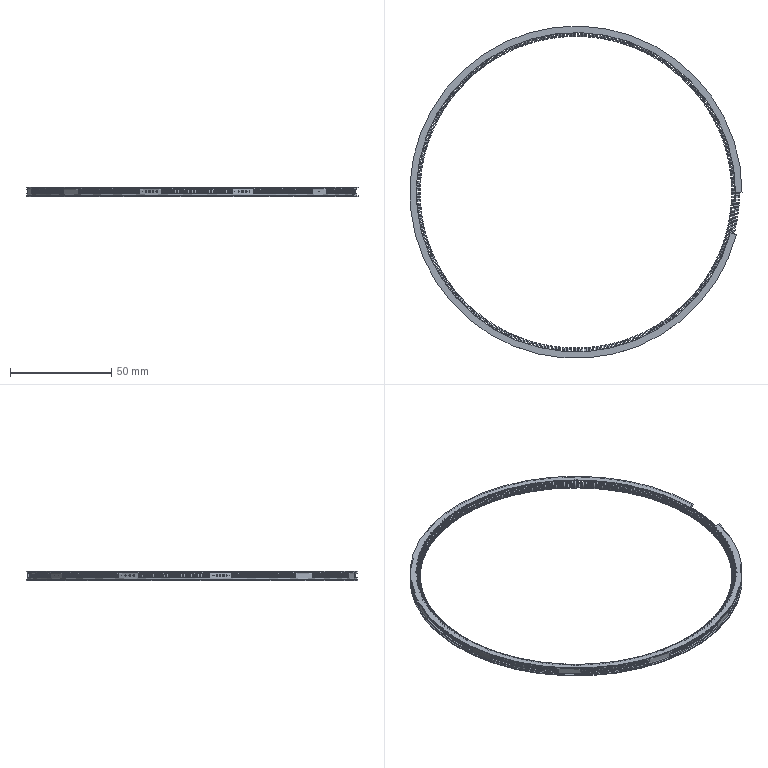Part | NX | features EXTRACT_STRING 371, Instance Feature 369, SWP104 362, EXTRACT_DATUM_AXIS 360, EXTRUDE 11, DATUM_CSYS 6, SKETCH 5, Pattern Feature 2 | 362 solids | 1500 faces | box 164 x 164 x 4.783 mm | volume 4407 mm3 | plane 769 | torus 722 | cylinder 6 | cone 3 | commonest cylinder face diameters 157.6 x2 163 x2 164 x2